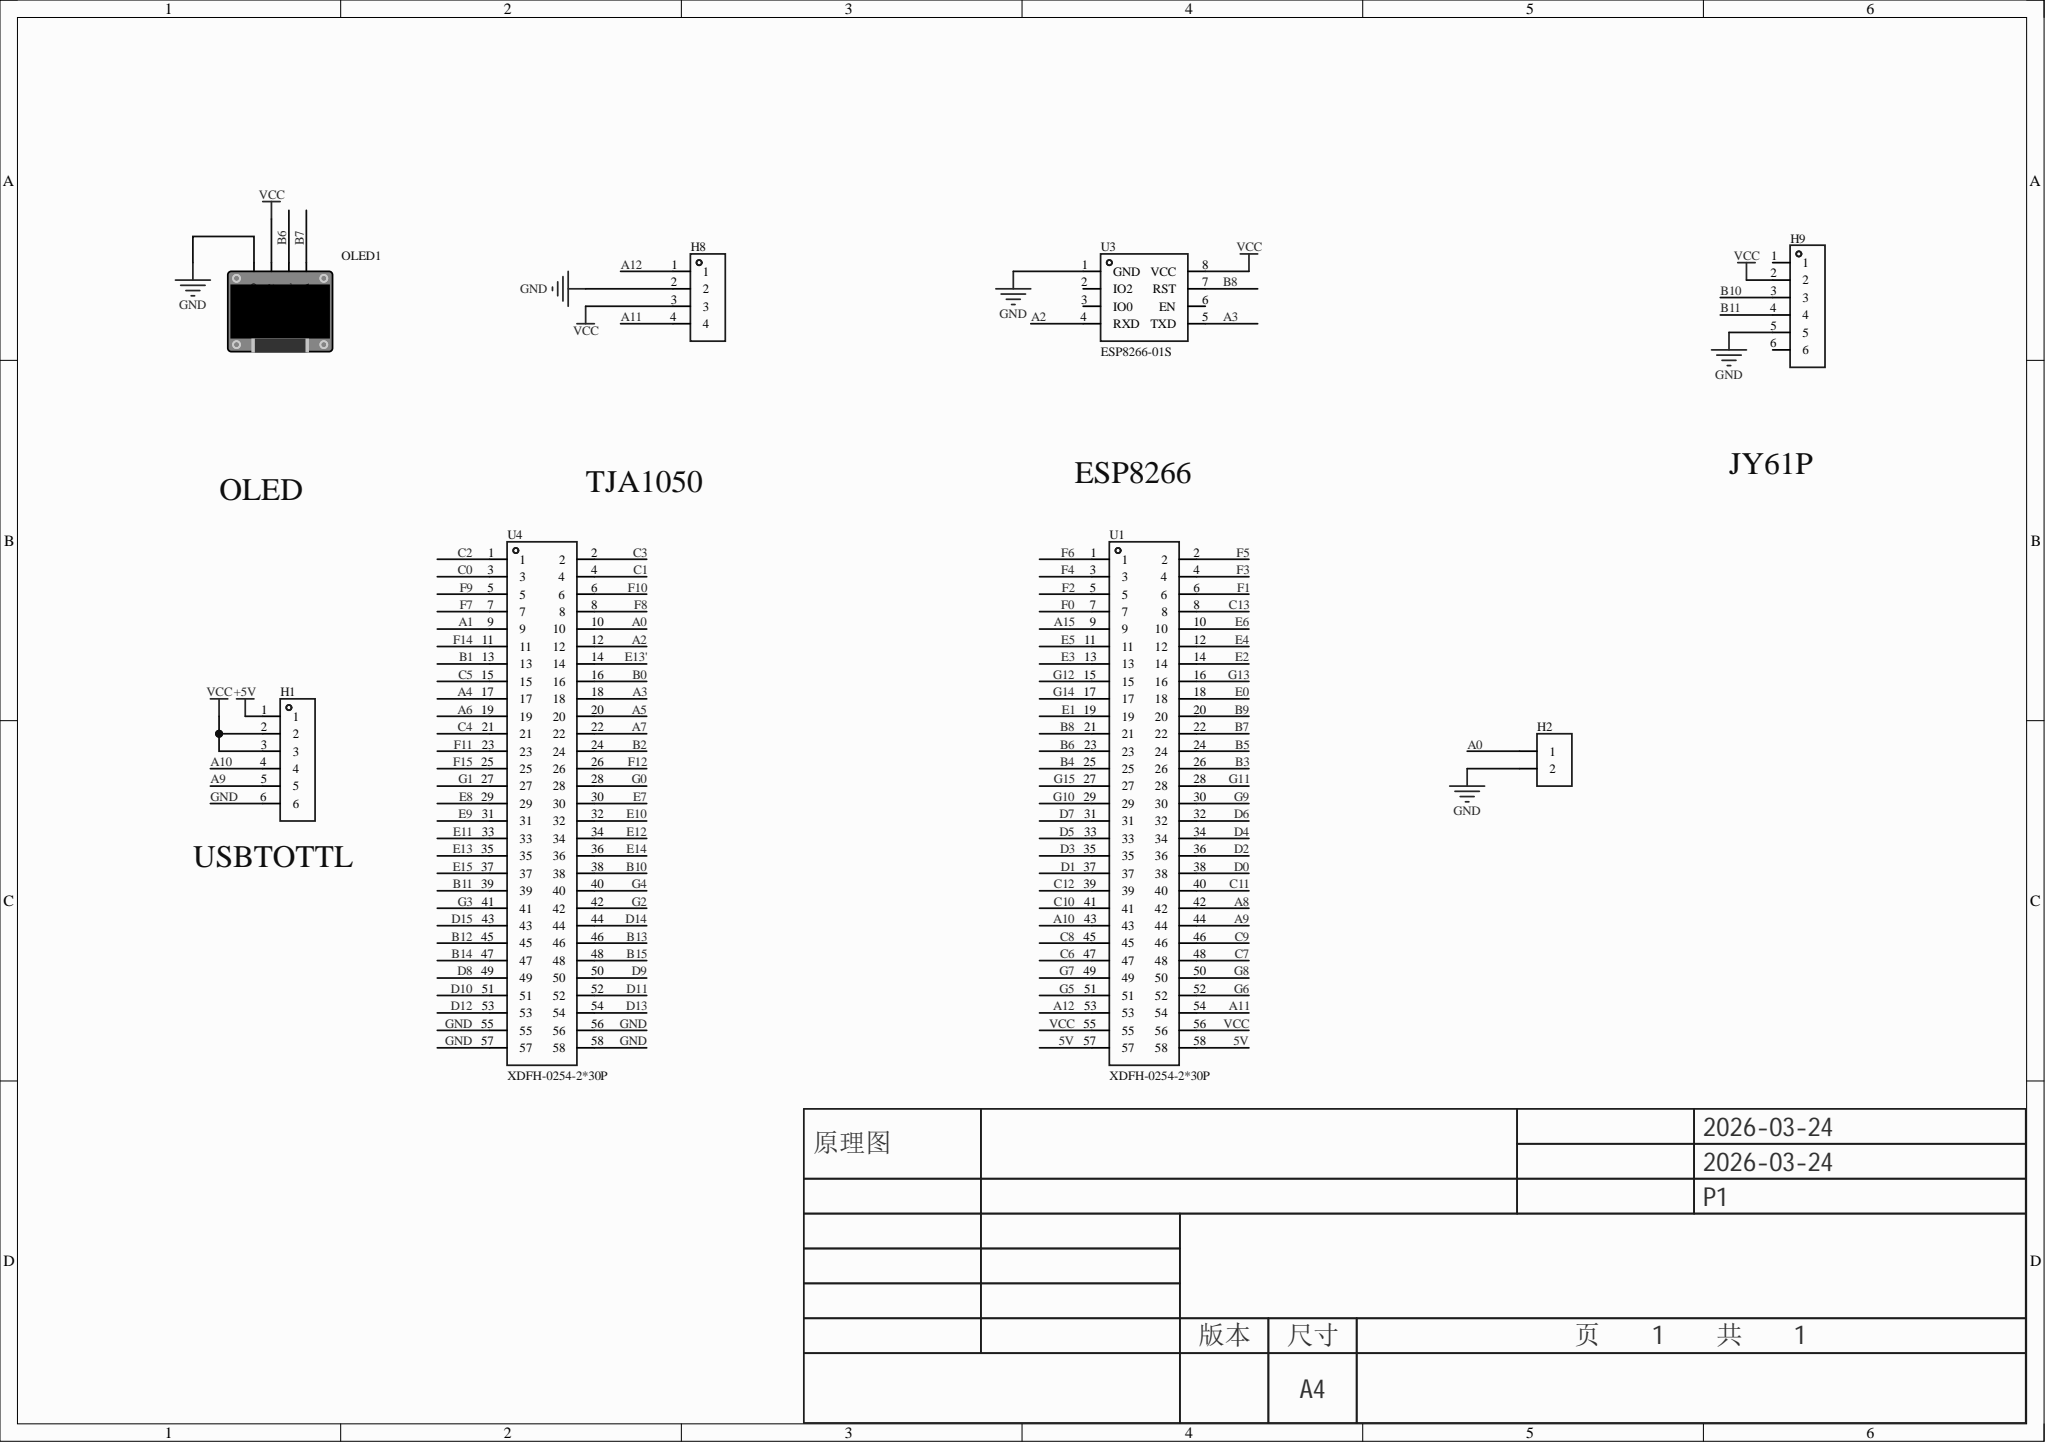Circuit board | Altium Designer | 8 parts | 15 nets
Bill of materials:
Comment,Description,Designator,Footprint,LibRef,Quantity
"","","H1, H9","HDR-TH_6P-P2.54-V-F","HDR-F_2.54_1x6P","2"
"","","H2","HDR-TH_2P-P2.54-V-F","HDR-F_2.54_1x2P","1"
"","","H8","HDR-TH_4P-P2.54-V-F","HDR-F_2.54_1x4P","1"
"","","OLED1","0.96OLED_4P","0.96OLED模块_4P","1"
"XDFH-0254-2*30P","连接器类型:简牛座;间距:2.54mm;结构:2x30P;额定电流:3A;额定电压:500V;封装形式:直插;排数:2;每排PIN数:30;触头材质:铜;触头镀层:金;工作温度范围:-45℃~+105℃;焊接温度(最大值):260℃;","U1, U4","CONN-TH_60P-P2.54_LX_XDFH-0254-2X30P","XDFH-0254-2*30P","2"
"ESP8266-01S","","U3","WIFIM-TH_ESP8266-01S","ESP8266-01S","1"
Netlist (Protel format):
[
H1
HDR-TH_6P-P2.54-V-F




]
[
H2
HDR-TH_2P-P2.54-V-F




]
[
H8
HDR-TH_4P-P2.54-V-F




]
[
H9
HDR-TH_6P-P2.54-V-F




]
[
OLED1
0.96OLED_4P




]
[
U1
CONN-TH_60P-P2.54_LX_XDFH-0254-2X30P
XDFH-0254-2*30P



]
[
U3
WIFIM-TH_ESP8266-01S
ESP8266-01S



]
[
U4
CONN-TH_60P-P2.54_LX_XDFH-0254-2X30P
XDFH-0254-2*30P



]
(
VCC
H1-2
H1-3
H8-3
H9-2
OLED1-2
U1-55
U1-56
U3-8
)
(
GND
H1-6
H2-2
H8-2
H9-5
OLED1-1
U3-1
U4-55
U4-56
U4-57
U4-58
)
(
B11
H9-4
U4-39
)
(
B10
H9-3
U4-38
)
(
B8
U1-21
U3-7
)
(
B7
OLED1-4
U1-22
)
(
B6
OLED1-3
U1-23
)
(
A12
H8-1
U1-53
)
(
A11
H8-4
U1-54
)
(
A10
H1-4
U1-43
)
(
A9
H1-5
U1-44
)
(
A3
U3-5
U4-18
)
(
A2
U3-4
U4-12
)
(
A0
H2-1
U4-10
)
(
5V
U1-57
U1-58
)